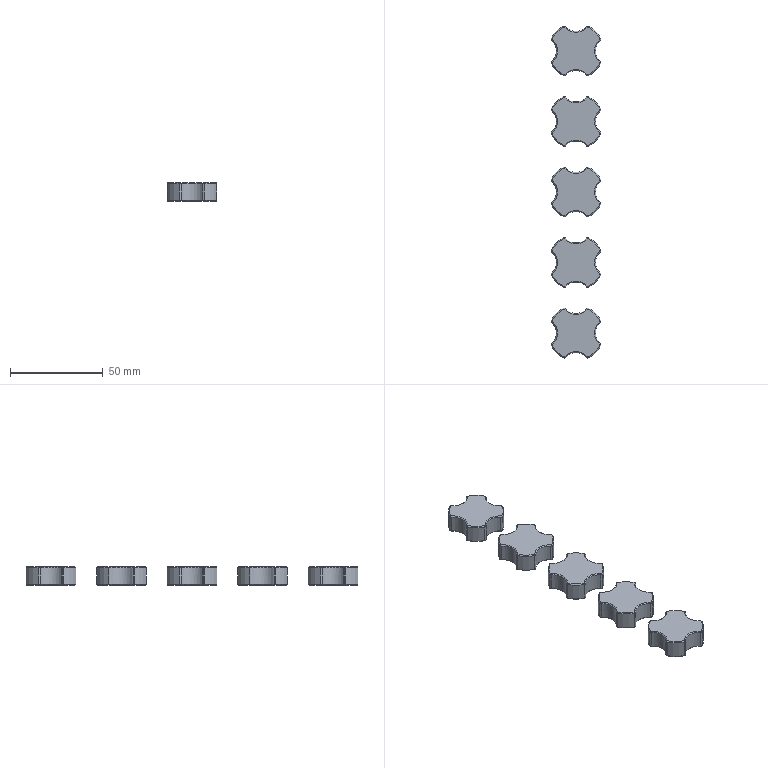Part | 5 solids | 325 faces | box 26.875 x 178.875 x 10 mm | volume 27042 mm3 | cone 210 | cylinder 105 | plane 10 | commonest cylinder face diameters 2 x50 15 x25 30 x20 4 x10